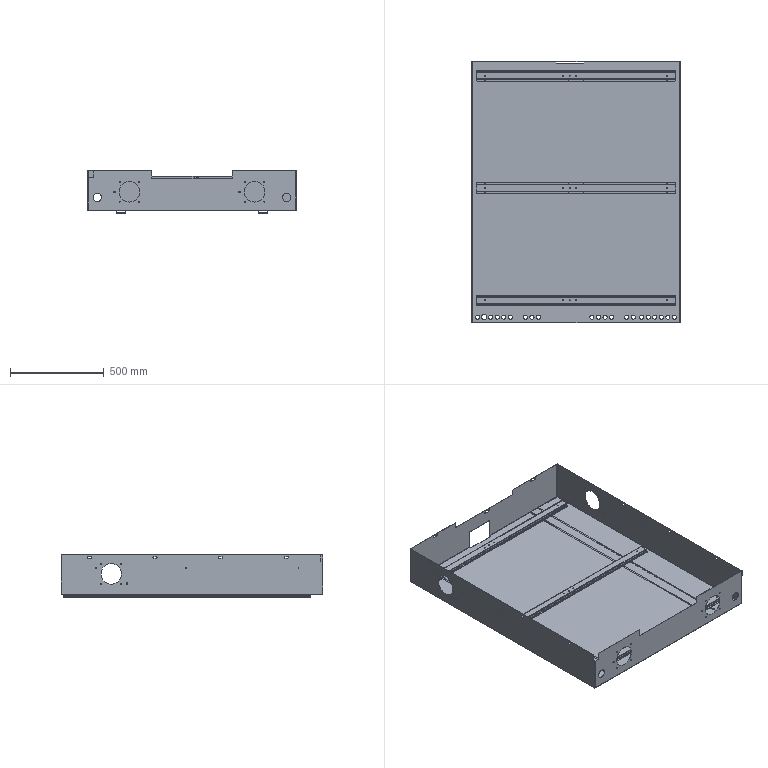Part | SolidWorks | features LayoutProfileFeature 1 | 6 solids | 536 faces | box 1110 x 1395 x 228 mm | volume 4724394 mm3 | cylinder 306 | plane 220 | spline 10 | commonest cylinder face diameters 3 x48 22 x40 4.2 x30 4 x29 10 x24 1.473 x20